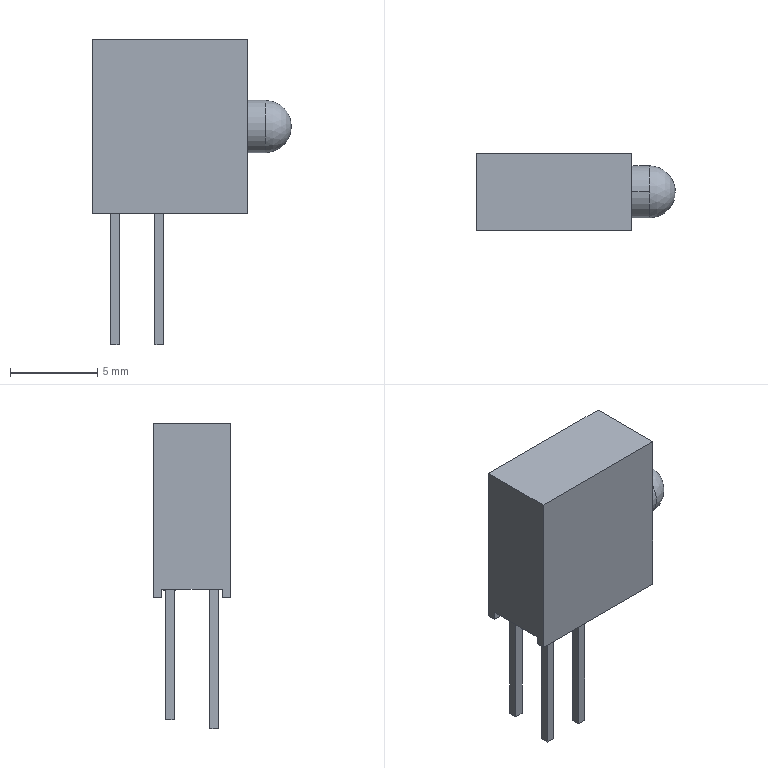Part | SolidWorks | features BaseBody 1 | 1 solid | 39 faces | box 11.4 x 4.45 x 17.5 mm | volume 402.599 mm3 | plane 34 | cylinder 4 | sphere 1 | commonest cylinder face diameters 0.707 x2 3 x2
STEP:
#1=CARTESIAN_POINT('',(107.207,42.288,40.));
#2=VERTEX_POINT('',#1);
#3=CARTESIAN_POINT('',(107.207,42.288,43.));
#4=VERTEX_POINT('',#3);
#5=CARTESIAN_POINT('',(107.207,42.288,41.5));
#6=DIRECTION('',(1.,0.,0.));
#7=DIRECTION('',(0.,0.,-1.));
#8=AXIS2_PLACEMENT_3D('',#5,#6,#7);
#9=CIRCLE('',#8,1.5);
#10=EDGE_CURVE('',#2,#4,#9,.T.);
#11=ORIENTED_EDGE('',*,*,#10,.T.);
#12=CARTESIAN_POINT('',(108.207,42.288,43.));
#13=VERTEX_POINT('',#12);
#14=CARTESIAN_POINT('',(109.807,42.288,43.));
#15=DIRECTION('',(1.,0.,0.));
#16=VECTOR('',#15,1000.);
#17=LINE('',#14,#16);
#18=EDGE_CURVE('',#4,#13,#17,.T.);
#19=ORIENTED_EDGE('',*,*,#18,.T.);
#20=CARTESIAN_POINT('',(108.207,42.288,40.));
#21=VERTEX_POINT('',#20);
#22=CARTESIAN_POINT('',(108.207,42.288,41.5));
#23=DIRECTION('',(-1.,0.,0.));
#24=DIRECTION('',(0.,0.,-1.));
#25=AXIS2_PLACEMENT_3D('',#22,#23,#24);
#26=CIRCLE('',#25,1.5);
#27=EDGE_CURVE('',#13,#21,#26,.T.);
#28=ORIENTED_EDGE('',*,*,#27,.T.);
#29=CARTESIAN_POINT('',(109.807,42.288,40.));
#30=DIRECTION('',(1.,0.,0.));
#31=VECTOR('',#30,1000.);
#32=LINE('',#29,#31);
#33=EDGE_CURVE('',#2,#21,#32,.T.);
#34=ORIENTED_EDGE('',*,*,#33,.F.);
#35=EDGE_LOOP('',(#11,#19,#28,#34));
#36=FACE_OUTER_BOUND('',#35,.T.);
#37=CARTESIAN_POINT('',(109.807,42.288,41.5));
#38=DIRECTION('',(1.,0.,0.));
#39=DIRECTION('',(0.,0.,-1.));
#40=AXIS2_PLACEMENT_3D('',#37,#38,#39);
#41=CYLINDRICAL_SURFACE('',#40,1.5);
#42=ADVANCED_FACE('',(#36),#41,.T.);
#43=CARTESIAN_POINT('',(102.481,43.558,37.));
#44=VERTEX_POINT('',#43);
#45=CARTESIAN_POINT('',(101.774,43.558,37.));
#46=VERTEX_POINT('',#45);
#47=CARTESIAN_POINT('',(102.127,43.558,37.));
#48=DIRECTION('',(0.,0.,1.));
#49=DIRECTION('',(-1.,0.,0.));
#50=AXIS2_PLACEMENT_3D('',#47,#48,#49);
#51=CIRCLE('',#50,0.3536);
#52=EDGE_CURVE('',#44,#46,#51,.T.);
#53=ORIENTED_EDGE('',*,*,#52,.F.);
#54=CARTESIAN_POINT('',(102.481,43.558,36.9));
#55=VERTEX_POINT('',#54);
#56=CARTESIAN_POINT('',(102.481,43.558,37.));
#57=DIRECTION('',(0.,0.,-1.));
#58=VECTOR('',#57,1000.);
#59=LINE('',#56,#58);
#60=EDGE_CURVE('',#44,#55,#59,.T.);
#61=ORIENTED_EDGE('',*,*,#60,.T.);
#62=CARTESIAN_POINT('',(102.377,43.808,36.9));
#63=VERTEX_POINT('',#62);
#64=CARTESIAN_POINT('',(102.127,43.558,36.9));
#65=DIRECTION('',(0.,0.,1.));
#66=DIRECTION('',(-1.,0.,0.));
#67=AXIS2_PLACEMENT_3D('',#64,#65,#66);
#68=CIRCLE('',#67,0.3536);
#69=EDGE_CURVE('',#55,#63,#68,.T.);
#70=ORIENTED_EDGE('',*,*,#69,.T.);
#71=CARTESIAN_POINT('',(101.877,43.808,36.9));
#72=VERTEX_POINT('',#71);
#73=CARTESIAN_POINT('',(102.127,43.558,36.9));
#74=DIRECTION('',(0.,0.,1.));
#75=DIRECTION('',(-1.,0.,0.));
#76=AXIS2_PLACEMENT_3D('',#73,#74,#75);
#77=CIRCLE('',#76,0.3536);
#78=EDGE_CURVE('',#63,#72,#77,.T.);
#79=ORIENTED_EDGE('',*,*,#78,.T.);
#80=CARTESIAN_POINT('',(101.774,43.558,36.9));
#81=VERTEX_POINT('',#80);
#82=CARTESIAN_POINT('',(102.127,43.558,36.9));
#83=DIRECTION('',(0.,0.,1.));
#84=DIRECTION('',(-1.,0.,0.));
#85=AXIS2_PLACEMENT_3D('',#82,#83,#84);
#86=CIRCLE('',#85,0.3536);
#87=EDGE_CURVE('',#72,#81,#86,.T.);
#88=ORIENTED_EDGE('',*,*,#87,.T.);
#89=CARTESIAN_POINT('',(101.774,43.558,37.));
#90=DIRECTION('',(0.,0.,-1.));
#91=VECTOR('',#90,1000.);
#92=LINE('',#89,#91);
#93=EDGE_CURVE('',#46,#81,#92,.T.);
#94=ORIENTED_EDGE('',*,*,#93,.F.);
#95=EDGE_LOOP('',(#53,#61,#70,#79,#88,#94));
#96=FACE_OUTER_BOUND('',#95,.T.);
#97=CARTESIAN_POINT('',(102.127,43.558,37.));
#98=DIRECTION('',(0.,0.,-1.));
#99=DIRECTION('',(-1.,0.,0.));
#100=AXIS2_PLACEMENT_3D('',#97,#98,#99);
#101=CYLINDRICAL_SURFACE('',#100,0.3536);
#102=ADVANCED_FACE('',(#96),#101,.T.);
#103=CARTESIAN_POINT('',(98.307,44.513,36.5));
#104=VERTEX_POINT('',#103);
#105=CARTESIAN_POINT('',(98.307,44.513,46.5));
#106=VERTEX_POINT('',#105);
#107=CARTESIAN_POINT('',(98.307,44.513,36.5));
#108=DIRECTION('',(0.,0.,1.));
#109=VECTOR('',#108,1000.);
#110=LINE('',#107,#109);
#111=EDGE_CURVE('',#104,#106,#110,.T.);
#112=ORIENTED_EDGE('',*,*,#111,.T.);
#113=CARTESIAN_POINT('',(107.207,44.513,46.5));
#114=VERTEX_POINT('',#113);
#115=CARTESIAN_POINT('',(98.307,44.513,46.5));
#116=DIRECTION('',(1.,0.,0.));
#117=VECTOR('',#116,1000.);
#118=LINE('',#115,#117);
#119=EDGE_CURVE('',#106,#114,#118,.T.);
#120=ORIENTED_EDGE('',*,*,#119,.T.);
#121=CARTESIAN_POINT('',(107.207,44.513,36.5));
#122=VERTEX_POINT('',#121);
#123=CARTESIAN_POINT('',(107.207,44.513,36.5));
#124=DIRECTION('',(0.,0.,-1.));
#125=VECTOR('',#124,1000.);
#126=LINE('',#123,#125);
#127=EDGE_CURVE('',#114,#122,#126,.T.);
#128=ORIENTED_EDGE('',*,*,#127,.T.);
#129=CARTESIAN_POINT('',(98.307,44.513,36.5));
#130=DIRECTION('',(-1.,0.,0.));
#131=VECTOR('',#130,1000.);
#132=LINE('',#129,#131);
#133=EDGE_CURVE('',#122,#104,#132,.T.);
#134=ORIENTED_EDGE('',*,*,#133,.T.);
#135=EDGE_LOOP('',(#112,#120,#128,#134));
#136=FACE_OUTER_BOUND('',#135,.T.);
#137=CARTESIAN_POINT('',(98.307,44.513,36.5));
#138=DIRECTION('',(0.,1.,0.));
#139=DIRECTION('',(0.,0.,1.));
#140=AXIS2_PLACEMENT_3D('',#137,#138,#139);
#141=PLANE('',#140);
#142=ADVANCED_FACE('',(#136),#141,.T.);
#143=ORIENTED_EDGE('',*,*,#119,.F.);
#144=CARTESIAN_POINT('',(98.307,40.063,46.5));
#145=VERTEX_POINT('',#144);
#146=CARTESIAN_POINT('',(98.307,44.513,46.5));
#147=DIRECTION('',(0.,1.,0.));
#148=VECTOR('',#147,1000.);
#149=LINE('',#146,#148);
#150=EDGE_CURVE('',#145,#106,#149,.T.);
#151=ORIENTED_EDGE('',*,*,#150,.F.);
#152=CARTESIAN_POINT('',(107.207,40.063,46.5));
#153=VERTEX_POINT('',#152);
#154=CARTESIAN_POINT('',(98.307,40.063,46.5));
#155=DIRECTION('',(-1.,0.,0.));
#156=VECTOR('',#155,1000.);
#157=LINE('',#154,#156);
#158=EDGE_CURVE('',#153,#145,#157,.T.);
#159=ORIENTED_EDGE('',*,*,#158,.F.);
#160=CARTESIAN_POINT('',(107.207,44.513,46.5));
#161=DIRECTION('',(0.,-1.,0.));
#162=VECTOR('',#161,1000.);
#163=LINE('',#160,#162);
#164=EDGE_CURVE('',#114,#153,#163,.T.);
#165=ORIENTED_EDGE('',*,*,#164,.F.);
#166=EDGE_LOOP('',(#143,#151,#159,#165));
#167=FACE_OUTER_BOUND('',#166,.T.);
#168=CARTESIAN_POINT('',(98.307,44.513,46.5));
#169=DIRECTION('',(0.,0.,-1.));
#170=DIRECTION('',(-1.,0.,0.));
#171=AXIS2_PLACEMENT_3D('',#168,#169,#170);
#172=PLANE('',#171);
#173=ADVANCED_FACE('',(#167),#172,.F.);
#174=CARTESIAN_POINT('',(98.307,40.063,36.5));
#175=VERTEX_POINT('',#174);
#176=CARTESIAN_POINT('',(98.307,40.063,36.5));
#177=DIRECTION('',(0.,0.,-1.));
#178=VECTOR('',#177,1000.);
#179=LINE('',#176,#178);
#180=EDGE_CURVE('',#145,#175,#179,.T.);
#181=ORIENTED_EDGE('',*,*,#180,.F.);
#182=ORIENTED_EDGE('',*,*,#150,.T.);
#183=ORIENTED_EDGE('',*,*,#111,.F.);
#184=CARTESIAN_POINT('',(98.307,44.013,36.5));
#185=VERTEX_POINT('',#184);
#186=CARTESIAN_POINT('',(98.307,44.513,36.5));
#187=DIRECTION('',(0.,1.,0.));
#188=VECTOR('',#187,1000.);
#189=LINE('',#186,#188);
#190=EDGE_CURVE('',#185,#104,#189,.T.);
#191=ORIENTED_EDGE('',*,*,#190,.F.);
#192=CARTESIAN_POINT('',(98.307,44.013,37.));
#193=VERTEX_POINT('',#192);
#194=CARTESIAN_POINT('',(98.307,44.013,37.));
#195=DIRECTION('',(0.,0.,-1.));
#196=VECTOR('',#195,1000.);
#197=LINE('',#194,#196);
#198=EDGE_CURVE('',#193,#185,#197,.T.);
#199=ORIENTED_EDGE('',*,*,#198,.F.);
#200=CARTESIAN_POINT('',(98.307,40.563,37.));
#201=VERTEX_POINT('',#200);
#202=CARTESIAN_POINT('',(98.307,44.513,37.));
#203=DIRECTION('',(0.,1.,0.));
#204=VECTOR('',#203,1000.);
#205=LINE('',#202,#204);
#206=EDGE_CURVE('',#201,#193,#205,.T.);
#207=ORIENTED_EDGE('',*,*,#206,.F.);
#208=CARTESIAN_POINT('',(98.307,40.563,36.5));
#209=VERTEX_POINT('',#208);
#210=CARTESIAN_POINT('',(98.307,40.563,35.6));
#211=DIRECTION('',(0.,0.,1.));
#212=VECTOR('',#211,1000.);
#213=LINE('',#210,#212);
#214=EDGE_CURVE('',#209,#201,#213,.T.);
#215=ORIENTED_EDGE('',*,*,#214,.F.);
#216=CARTESIAN_POINT('',(98.307,44.513,36.5));
#217=DIRECTION('',(0.,-1.,0.));
#218=VECTOR('',#217,1000.);
#219=LINE('',#216,#218);
#220=EDGE_CURVE('',#209,#175,#219,.T.);
#221=ORIENTED_EDGE('',*,*,#220,.T.);
#222=EDGE_LOOP('',(#181,#182,#183,#191,#199,#207,#215,#221));
#223=FACE_OUTER_BOUND('',#222,.T.);
#224=CARTESIAN_POINT('',(98.307,44.513,36.5));
#225=DIRECTION('',(1.,0.,0.));
#226=DIRECTION('',(0.,0.,-1.));
#227=AXIS2_PLACEMENT_3D('',#224,#225,#226);
#228=PLANE('',#227);
#229=ADVANCED_FACE('',(#223),#228,.F.);
#230=ORIENTED_EDGE('',*,*,#133,.F.);
#231=CARTESIAN_POINT('',(107.207,44.013,36.5));
#232=VERTEX_POINT('',#231);
#233=CARTESIAN_POINT('',(107.207,44.513,36.5));
#234=DIRECTION('',(0.,1.,0.));
#235=VECTOR('',#234,1000.);
#236=LINE('',#233,#235);
#237=EDGE_CURVE('',#232,#122,#236,.T.);
#238=ORIENTED_EDGE('',*,*,#237,.F.);
#239=CARTESIAN_POINT('',(107.207,44.013,36.5));
#240=DIRECTION('',(1.,0.,0.));
#241=VECTOR('',#240,1000.);
#242=LINE('',#239,#241);
#243=EDGE_CURVE('',#185,#232,#242,.T.);
#244=ORIENTED_EDGE('',*,*,#243,.F.);
#245=ORIENTED_EDGE('',*,*,#190,.T.);
#246=EDGE_LOOP('',(#230,#238,#244,#245));
#247=FACE_OUTER_BOUND('',#246,.T.);
#248=CARTESIAN_POINT('',(107.207,44.513,36.5));
#249=DIRECTION('',(0.,0.,1.));
#250=DIRECTION('',(1.,0.,0.));
#251=AXIS2_PLACEMENT_3D('',#248,#249,#250);
#252=PLANE('',#251);
#253=ADVANCED_FACE('',(#247),#252,.F.);
#254=ORIENTED_EDGE('',*,*,#10,.F.);
#255=CARTESIAN_POINT('',(107.207,42.288,41.5));
#256=DIRECTION('',(1.,0.,0.));
#257=DIRECTION('',(0.,0.,-1.));
#258=AXIS2_PLACEMENT_3D('',#255,#256,#257);
#259=CIRCLE('',#258,1.5);
#260=EDGE_CURVE('',#4,#2,#259,.T.);
#261=ORIENTED_EDGE('',*,*,#260,.F.);
#262=EDGE_LOOP('',(#254,#261));
#263=FACE_BOUND('',#262,.T.);
#264=CARTESIAN_POINT('',(107.207,40.063,36.5));
#265=VERTEX_POINT('',#264);
#266=CARTESIAN_POINT('',(107.207,40.063,46.5));
#267=DIRECTION('',(0.,0.,1.));
#268=VECTOR('',#267,1000.);
#269=LINE('',#266,#268);
#270=EDGE_CURVE('',#265,#153,#269,.T.);
#271=ORIENTED_EDGE('',*,*,#270,.F.);
#272=CARTESIAN_POINT('',(107.207,40.563,36.5));
#273=VERTEX_POINT('',#272);
#274=CARTESIAN_POINT('',(107.207,44.513,36.5));
#275=DIRECTION('',(0.,1.,0.));
#276=VECTOR('',#275,1000.);
#277=LINE('',#274,#276);
#278=EDGE_CURVE('',#265,#273,#277,.T.);
#279=ORIENTED_EDGE('',*,*,#278,.T.);
#280=CARTESIAN_POINT('',(107.207,40.563,37.));
#281=VERTEX_POINT('',#280);
#282=CARTESIAN_POINT('',(107.207,40.563,35.6));
#283=DIRECTION('',(0.,0.,-1.));
#284=VECTOR('',#283,1000.);
#285=LINE('',#282,#284);
#286=EDGE_CURVE('',#281,#273,#285,.T.);
#287=ORIENTED_EDGE('',*,*,#286,.F.);
#288=CARTESIAN_POINT('',(107.207,44.013,37.));
#289=VERTEX_POINT('',#288);
#290=CARTESIAN_POINT('',(107.207,44.513,37.));
#291=DIRECTION('',(0.,-1.,0.));
#292=VECTOR('',#291,1000.);
#293=LINE('',#290,#292);
#294=EDGE_CURVE('',#289,#281,#293,.T.);
#295=ORIENTED_EDGE('',*,*,#294,.F.);
#296=CARTESIAN_POINT('',(107.207,44.013,46.5));
#297=DIRECTION('',(0.,0.,1.));
#298=VECTOR('',#297,1000.);
#299=LINE('',#296,#298);
#300=EDGE_CURVE('',#232,#289,#299,.T.);
#301=ORIENTED_EDGE('',*,*,#300,.F.);
#302=ORIENTED_EDGE('',*,*,#237,.T.);
#303=ORIENTED_EDGE('',*,*,#127,.F.);
#304=ORIENTED_EDGE('',*,*,#164,.T.);
#305=EDGE_LOOP('',(#271,#279,#287,#295,#301,#302,#303,#304));
#306=FACE_OUTER_BOUND('',#305,.T.);
#307=CARTESIAN_POINT('',(107.207,44.513,46.5));
#308=DIRECTION('',(-1.,0.,0.));
#309=DIRECTION('',(0.,0.,1.));
#310=AXIS2_PLACEMENT_3D('',#307,#308,#309);
#311=PLANE('',#310);
#312=ADVANCED_FACE('',(#263,#306),#311,.F.);
#313=ORIENTED_EDGE('',*,*,#270,.T.);
#314=ORIENTED_EDGE('',*,*,#158,.T.);
#315=ORIENTED_EDGE('',*,*,#180,.T.);
#316=CARTESIAN_POINT('',(98.307,40.063,36.5));
#317=DIRECTION('',(-1.,0.,0.));
#318=VECTOR('',#317,1000.);
#319=LINE('',#316,#318);
#320=EDGE_CURVE('',#265,#175,#319,.T.);
#321=ORIENTED_EDGE('',*,*,#320,.F.);
#322=EDGE_LOOP('',(#313,#314,#315,#321));
#323=FACE_OUTER_BOUND('',#322,.T.);
#324=CARTESIAN_POINT('',(98.307,40.063,36.5));
#325=DIRECTION('',(0.,1.,0.));
#326=DIRECTION('',(0.,0.,1.));
#327=AXIS2_PLACEMENT_3D('',#324,#325,#326);
#328=PLANE('',#327);
#329=ADVANCED_FACE('',(#323),#328,.F.);
#330=CARTESIAN_POINT('',(102.127,43.558,37.));
#331=DIRECTION('',(0.,0.,1.));
#332=DIRECTION('',(-1.,0.,0.));
#333=AXIS2_PLACEMENT_3D('',#330,#331,#332);
#334=CIRCLE('',#333,0.3536);
#335=EDGE_CURVE('',#46,#44,#334,.T.);
#336=ORIENTED_EDGE('',*,*,#335,.T.);
#337=ORIENTED_EDGE('',*,*,#52,.T.);
#338=EDGE_LOOP('',(#336,#337));
#339=FACE_BOUND('',#338,.T.);
#340=CARTESIAN_POINT('',(99.837,43.808,37.));
#341=VERTEX_POINT('',#340);
#342=CARTESIAN_POINT('',(99.837,43.308,37.));
#343=VERTEX_POINT('',#342);
#344=CARTESIAN_POINT('',(99.837,43.808,37.));
#345=DIRECTION('',(0.,-1.,0.));
#346=VECTOR('',#345,1000.);
#347=LINE('',#344,#346);
#348=EDGE_CURVE('',#341,#343,#347,.T.);
#349=ORIENTED_EDGE('',*,*,#348,.F.);
#350=CARTESIAN_POINT('',(99.337,43.808,37.));
#351=VERTEX_POINT('',#350);
#352=CARTESIAN_POINT('',(92.707,43.808,37.));
#353=DIRECTION('',(-1.,0.,0.));
#354=VECTOR('',#353,1000.);
#355=LINE('',#352,#354);
#356=EDGE_CURVE('',#341,#351,#355,.T.);
#357=ORIENTED_EDGE('',*,*,#356,.T.);
#358=CARTESIAN_POINT('',(99.337,43.308,37.));
#359=VERTEX_POINT('',#358);
#360=CARTESIAN_POINT('',(99.337,43.558,37.));
#361=DIRECTION('',(0.,1.,0.));
#362=VECTOR('',#361,1000.);
#363=LINE('',#360,#362);
#364=EDGE_CURVE('',#359,#351,#363,.T.);
#365=ORIENTED_EDGE('',*,*,#364,.F.);
#366=CARTESIAN_POINT('',(100.857,43.308,37.));
#367=DIRECTION('',(-1.,0.,0.));
#368=VECTOR('',#367,1000.);
#369=LINE('',#366,#368);
#370=EDGE_CURVE('',#343,#359,#369,.T.);
#371=ORIENTED_EDGE('',*,*,#370,.F.);
#372=EDGE_LOOP('',(#349,#357,#365,#371));
#373=FACE_BOUND('',#372,.T.);
#374=CARTESIAN_POINT('',(99.837,41.268,37.));
#375=VERTEX_POINT('',#374);
#376=CARTESIAN_POINT('',(99.837,40.768,37.));
#377=VERTEX_POINT('',#376);
#378=CARTESIAN_POINT('',(99.837,41.268,37.));
#379=DIRECTION('',(0.,-1.,0.));
#380=VECTOR('',#379,1000.);
#381=LINE('',#378,#380);
#382=EDGE_CURVE('',#375,#377,#381,.T.);
#383=ORIENTED_EDGE('',*,*,#382,.F.);
#384=CARTESIAN_POINT('',(99.337,41.268,37.));
#385=VERTEX_POINT('',#384);
#386=CARTESIAN_POINT('',(92.707,41.268,37.));
#387=DIRECTION('',(-1.,0.,0.));
#388=VECTOR('',#387,1000.);
#389=LINE('',#386,#388);
#390=EDGE_CURVE('',#375,#385,#389,.T.);
#391=ORIENTED_EDGE('',*,*,#390,.T.);
#392=CARTESIAN_POINT('',(99.337,40.768,37.));
#393=VERTEX_POINT('',#392);
#394=CARTESIAN_POINT('',(99.337,41.268,37.));
#395=DIRECTION('',(0.,1.,0.));
#396=VECTOR('',#395,1000.);
#397=LINE('',#394,#396);
#398=EDGE_CURVE('',#393,#385,#397,.T.);
#399=ORIENTED_EDGE('',*,*,#398,.F.);
#400=CARTESIAN_POINT('',(98.307,40.768,37.));
#401=DIRECTION('',(-1.,0.,0.));
#402=VECTOR('',#401,1000.);
#403=LINE('',#400,#402);
#404=EDGE_CURVE('',#377,#393,#403,.T.);
#405=ORIENTED_EDGE('',*,*,#404,.F.);
#406=EDGE_LOOP('',(#383,#391,#399,#405));
#407=FACE_BOUND('',#406,.T.);
#408=ORIENTED_EDGE('',*,*,#206,.T.);
#409=CARTESIAN_POINT('',(92.707,44.013,37.));
#410=DIRECTION('',(1.,0.,0.));
#411=VECTOR('',#410,1000.);
#412=LINE('',#409,#411);
#413=EDGE_CURVE('',#193,#289,#412,.T.);
#414=ORIENTED_EDGE('',*,*,#413,.T.);
#415=ORIENTED_EDGE('',*,*,#294,.T.);
#416=CARTESIAN_POINT('',(92.707,40.563,37.));
#417=DIRECTION('',(-1.,0.,0.));
#418=VECTOR('',#417,1000.);
#419=LINE('',#416,#418);
#420=EDGE_CURVE('',#281,#201,#419,.T.);
#421=ORIENTED_EDGE('',*,*,#420,.T.);
#422=EDGE_LOOP('',(#408,#414,#415,#421));
#423=FACE_OUTER_BOUND('',#422,.T.);
#424=CARTESIAN_POINT('',(101.877,41.268,37.));
#425=VERTEX_POINT('',#424);
#426=CARTESIAN_POINT('',(102.377,41.268,37.));
#427=VERTEX_POINT('',#426);
#428=CARTESIAN_POINT('',(98.307,41.268,37.));
#429=DIRECTION('',(1.,0.,0.));
#430=VECTOR('',#429,1000.);
#431=LINE('',#428,#430);
#432=EDGE_CURVE('',#425,#427,#431,.T.);
#433=ORIENTED_EDGE('',*,*,#432,.F.);
#434=CARTESIAN_POINT('',(101.877,40.768,37.));
#435=VERTEX_POINT('',#434);
#436=CARTESIAN_POINT('',(101.877,40.563,37.));
#437=DIRECTION('',(0.,-1.,0.));
#438=VECTOR('',#437,1000.);
#439=LINE('',#436,#438);
#440=EDGE_CURVE('',#425,#435,#439,.T.);
#441=ORIENTED_EDGE('',*,*,#440,.T.);
#442=CARTESIAN_POINT('',(102.377,40.768,37.));
#443=VERTEX_POINT('',#442);
#444=CARTESIAN_POINT('',(98.307,40.768,37.));
#445=DIRECTION('',(1.,0.,0.));
#446=VECTOR('',#445,1000.);
#447=LINE('',#444,#446);
#448=EDGE_CURVE('',#435,#443,#447,.T.);
#449=ORIENTED_EDGE('',*,*,#448,.T.);
#450=CARTESIAN_POINT('',(102.377,41.268,37.));
#451=DIRECTION('',(0.,1.,0.));
#452=VECTOR('',#451,1000.);
#453=LINE('',#450,#452);
#454=EDGE_CURVE('',#443,#427,#453,.T.);
#455=ORIENTED_EDGE('',*,*,#454,.T.);
#456=EDGE_LOOP('',(#433,#441,#449,#455));
#457=FACE_BOUND('',#456,.T.);
#458=CARTESIAN_POINT('',(92.707,40.563,37.));
#459=DIRECTION('',(0.,0.,-1.));
#460=DIRECTION('',(-1.,0.,0.));
#461=AXIS2_PLACEMENT_3D('',#458,#459,#460);
#462=PLANE('',#461);
#463=ADVANCED_FACE('',(#339,#373,#407,#423,#457),#462,.T.);
#464=ORIENTED_EDGE('',*,*,#198,.T.);
#465=ORIENTED_EDGE('',*,*,#243,.T.);
#466=ORIENTED_EDGE('',*,*,#300,.T.);
#467=ORIENTED_EDGE('',*,*,#413,.F.);
#468=EDGE_LOOP('',(#464,#465,#466,#467));
#469=FACE_OUTER_BOUND('',#468,.T.);
#470=CARTESIAN_POINT('',(92.707,44.013,37.));
#471=DIRECTION('',(0.,-1.,0.));
#472=DIRECTION('',(0.,0.,-1.));
#473=AXIS2_PLACEMENT_3D('',#470,#471,#472);
#474=PLANE('',#473);
#475=ADVANCED_FACE('',(#469),#474,.T.);
#476=ORIENTED_EDGE('',*,*,#18,.F.);
#477=ORIENTED_EDGE('',*,*,#260,.T.);
#478=ORIENTED_EDGE('',*,*,#33,.T.);
#479=CARTESIAN_POINT('',(108.207,42.288,41.5));
#480=DIRECTION('',(-1.,0.,0.));
#481=DIRECTION('',(0.,0.,-1.));
#482=AXIS2_PLACEMENT_3D('',#479,#480,#481);
#483=CIRCLE('',#482,1.5);
#484=EDGE_CURVE('',#21,#13,#483,.T.);
#485=ORIENTED_EDGE('',*,*,#484,.T.);
#486=EDGE_LOOP('',(#476,#477,#478,#485));
#487=FACE_OUTER_BOUND('',#486,.T.);
#488=CARTESIAN_POINT('',(109.807,42.288,41.5));
#489=DIRECTION('',(1.,0.,0.));
#490=DIRECTION('',(0.,0.,-1.));
#491=AXIS2_PLACEMENT_3D('',#488,#489,#490);
#492=CYLINDRICAL_SURFACE('',#491,1.5);
#493=ADVANCED_FACE('',(#487),#492,.T.);
#494=ORIENTED_EDGE('',*,*,#320,.T.);
#495=ORIENTED_EDGE('',*,*,#220,.F.);
#496=CARTESIAN_POINT('',(107.207,40.563,36.5));
#497=DIRECTION('',(-1.,0.,0.));
#498=VECTOR('',#497,1000.);
#499=LINE('',#496,#498);
#500=EDGE_CURVE('',#273,#209,#499,.T.);
#501=ORIENTED_EDGE('',*,*,#500,.F.);
#502=ORIENTED_EDGE('',*,*,#278,.F.);
#503=EDGE_LOOP('',(#494,#495,#501,#502));
#504=FACE_OUTER_BOUND('',#503,.T.);
#505=CARTESIAN_POINT('',(107.207,44.513,36.5));
#506=DIRECTION('',(0.,0.,1.));
#507=DIRECTION('',(1.,0.,0.));
#508=AXIS2_PLACEMENT_3D('',#505,#506,#507);
#509=PLANE('',#508);
#510=ADVANCED_FACE('',(#504),#509,.F.);
#511=ORIENTED_EDGE('',*,*,#60,.F.);
#512=ORIENTED_EDGE('',*,*,#335,.F.);
#513=ORIENTED_EDGE('',*,*,#93,.T.);
#514=CARTESIAN_POINT('',(101.877,43.308,36.9));
#515=VERTEX_POINT('',#514);
#516=CARTESIAN_POINT('',(102.127,43.558,36.9));
#517=DIRECTION('',(0.,0.,1.));
#518=DIRECTION('',(-1.,0.,0.));
#519=AXIS2_PLACEMENT_3D('',#516,#517,#518);
#520=CIRCLE('',#519,0.3536);
#521=EDGE_CURVE('',#81,#515,#520,.T.);
#522=ORIENTED_EDGE('',*,*,#521,.T.);
#523=CARTESIAN_POINT('',(102.377,43.308,36.9));
#524=VERTEX_POINT('',#523);
#525=CARTESIAN_POINT('',(102.127,43.558,36.9));
#526=DIRECTION('',(0.,0.,1.));
#527=DIRECTION('',(-1.,0.,0.));
#528=AXIS2_PLACEMENT_3D('',#525,#526,#527);
#529=CIRCLE('',#528,0.3536);
#530=EDGE_CURVE('',#515,#524,#529,.T.);
#531=ORIENTED_EDGE('',*,*,#530,.T.);
#532=CARTESIAN_POINT('',(102.127,43.558,36.9));
#533=DIRECTION('',(0.,0.,1.));
#534=DIRECTION('',(-1.,0.,0.));
#535=AXIS2_PLACEMENT_3D('',#532,#533,#534);
#536=CIRCLE('',#535,0.3536);
#537=EDGE_CURVE('',#524,#55,#536,.T.);
#538=ORIENTED_EDGE('',*,*,#537,.T.);
#539=EDGE_LOOP('',(#511,#512,#513,#522,#531,#538));
#540=FACE_OUTER_BOUND('',#539,.T.);
#541=CARTESIAN_POINT('',(102.127,43.558,37.));
#542=DIRECTION('',(0.,0.,-1.));
#543=DIRECTION('',(-1.,0.,0.));
#544=AXIS2_PLACEMENT_3D('',#541,#542,#543);
#545=CYLINDRICAL_SURFACE('',#544,0.3536);
#546=ADVANCED_FACE('',(#540),#545,.T.);
#547=CARTESIAN_POINT('',(99.837,43.808,29.5));
#548=VERTEX_POINT('',#547);
#549=CARTESIAN_POINT('',(99.837,43.808,28.5));
#550=DIRECTION('',(0.,0.,-1.));
#551=VECTOR('',#550,1000.);
#552=LINE('',#549,#551);
#553=EDGE_CURVE('',#341,#548,#552,.T.);
#554=ORIENTED_EDGE('',*,*,#553,.T.);
#555=CARTESIAN_POINT('',(99.337,43.808,29.5));
#556=VERTEX_POINT('',#555);
#557=CARTESIAN_POINT('',(100.857,43.808,29.5));
#558=DIRECTION('',(-1.,0.,0.));
#559=VECTOR('',#558,1000.);
#560=LINE('',#557,#559);
#561=EDGE_CURVE('',#548,#556,#560,.T.);
#562=ORIENTED_EDGE('',*,*,#561,.T.);
#563=CARTESIAN_POINT('',(99.337,43.808,28.5));
#564=DIRECTION('',(0.,0.,1.));
#565=VECTOR('',#564,1000.);
#566=LINE('',#563,#565);
#567=EDGE_CURVE('',#556,#351,#566,.T.);
#568=ORIENTED_EDGE('',*,*,#567,.T.);
#569=ORIENTED_EDGE('',*,*,#356,.F.);
#570=EDGE_LOOP('',(#554,#562,#568,#569));
#571=FACE_OUTER_BOUND('',#570,.T.);
#572=CARTESIAN_POINT('',(100.857,43.808,28.5));
#573=DIRECTION('',(0.,1.,0.));
#574=DIRECTION('',(0.,0.,1.));
#575=AXIS2_PLACEMENT_3D('',#572,#573,#574);
#576=PLANE('',#575);
#577=ADVANCED_FACE('',(#571),#576,.T.);
#578=CARTESIAN_POINT('',(99.337,41.268,29.));
#579=VERTEX_POINT('',#578);
#580=CARTESIAN_POINT('',(99.837,41.268,29.));
#581=VERTEX_POINT('',#580);
#582=CARTESIAN_POINT('',(98.307,41.268,29.));
#583=DIRECTION('',(1.,0.,0.));
#584=VECTOR('',#583,1000.);
#585=LINE('',#582,#584);
#586=EDGE_CURVE('',#579,#581,#585,.T.);
#587=ORIENTED_EDGE('',*,*,#586,.F.);
#588=CARTESIAN_POINT('',(99.337,41.268,36.5));
#589=DIRECTION('',(0.,0.,-1.));
#590=VECTOR('',#589,1000.);
#591=LINE('',#588,#590);
#592=EDGE_CURVE('',#385,#579,#591,.T.);
#593=ORIENTED_EDGE('',*,*,#592,.F.);
#594=ORIENTED_EDGE('',*,*,#390,.F.);
#595=CARTESIAN_POINT('',(99.837,41.268,36.5));
#596=DIRECTION('',(0.,0.,1.));
#597=VECTOR('',#596,1000.);
#598=LINE('',#595,#597);
#599=EDGE_CURVE('',#581,#375,#598,.T.);
#600=ORIENTED_EDGE('',*,*,#599,.F.);
#601=EDGE_LOOP('',(#587,#593,#594,#600));
#602=FACE_OUTER_BOUND('',#601,.T.);
#603=CARTESIAN_POINT('',(98.307,41.268,36.5));
#604=DIRECTION('',(0.,-1.,0.));
#605=DIRECTION('',(0.,0.,-1.));
#606=AXIS2_PLACEMENT_3D('',#603,#604,#605);
#607=PLANE('',#606);
#608=ADVANCED_FACE('',(#602),#607,.F.);
#609=ORIENTED_EDGE('',*,*,#214,.T.);
#610=ORIENTED_EDGE('',*,*,#420,.F.);
#611=ORIENTED_EDGE('',*,*,#286,.T.);
#612=ORIENTED_EDGE('',*,*,#500,.T.);
#613=EDGE_LOOP('',(#609,#610,#611,#612));
#614=FACE_OUTER_BOUND('',#613,.T.);
#615=CARTESIAN_POINT('',(92.707,40.563,35.6));
#616=DIRECTION('',(0.,1.,0.));
#617=DIRECTION('',(0.,0.,1.));
#618=AXIS2_PLACEMENT_3D('',#615,#616,#617);
#619=PLANE('',#618);
#620=ADVANCED_FACE('',(#614),#619,.T.);
#621=CARTESIAN_POINT('',(101.877,40.768,29.));
#622=VERTEX_POINT('',#621);
#623=CARTESIAN_POINT('',(101.877,41.268,29.));
#624=VERTEX_POINT('',#623);
#625=CARTESIAN_POINT('',(101.877,41.268,29.));
#626=DIRECTION('',(0.,1.,0.));
#627=VECTOR('',#626,1000.);
#628=LINE('',#625,#627);
#629=EDGE_CURVE('',#622,#624,#628,.T.);
#630=ORIENTED_EDGE('',*,*,#629,.F.);
#631=CARTESIAN_POINT('',(101.877,40.768,28.5));
#632=DIRECTION('',(0.,0.,-1.));
#633=VECTOR('',#632,1000.);
#634=LINE('',#631,#633);
#635=EDGE_CURVE('',#435,#622,#634,.T.);
#636=ORIENTED_EDGE('',*,*,#635,.F.);
#637=ORIENTED_EDGE('',*,*,#440,.F.);
#638=CARTESIAN_POINT('',(101.877,41.268,28.5));
#639=DIRECTION('',(0.,0.,1.));
#640=VECTOR('',#639,1000.);
#641=LINE('',#638,#640);
#642=EDGE_CURVE('',#624,#425,#641,.T.);
#643=ORIENTED_EDGE('',*,*,#642,.F.);
#644=EDGE_LOOP('',(#630,#636,#637,#643));
#645=FACE_OUTER_BOUND('',#644,.T.);
#646=CARTESIAN_POINT('',(101.877,41.268,28.5));
#647=DIRECTION('',(1.,0.,0.));
#648=DIRECTION('',(0.,0.,-1.));
#649=AXIS2_PLACEMENT_3D('',#646,#647,#648);
#650=PLANE('',#649);
#651=ADVANCED_FACE('',(#645),#650,.F.);
#652=ORIENTED_EDGE('',*,*,#484,.F.);
#653=ORIENTED_EDGE('',*,*,#27,.F.);
#654=EDGE_LOOP('',(#652,#653));
#655=FACE_OUTER_BOUND('',#654,.T.);
#656=CARTESIAN_POINT('',(108.207,42.288,41.5));
#657=DIRECTION('',(-1.,0.,0.));
#658=DIRECTION('',(0.,1.,0.));
#659=AXIS2_PLACEMENT_3D('',#656,#657,#658);
#660=SPHERICAL_SURFACE('',#659,1.5);
#661=ADVANCED_FACE('',(#655),#660,.T.);
#662=CARTESIAN_POINT('',(101.877,43.558,36.9));
#663=DIRECTION('',(0.,-1.,0.));
#664=VECTOR('',#663,1000.);
#665=LINE('',#662,#664);
#666=EDGE_CURVE('',#72,#515,#665,.T.);
#667=ORIENTED_EDGE('',*,*,#666,.T.);
#668=ORIENTED_EDGE('',*,*,#521,.F.);
#669=ORIENTED_EDGE('',*,*,#87,.F.);
#670=EDGE_LOOP('',(#667,#668,#669));
#671=FACE_OUTER_BOUND('',#670,.T.);
#672=CARTESIAN_POINT('',(102.127,43.558,36.9));
#673=DIRECTION('',(0.,0.,-1.));
#674=DIRECTION('',(-1.,0.,0.));
#675=AXIS2_PLACEMENT_3D('',#672,#673,#674);
#676=PLANE('',#675);
#677=ADVANCED_FACE('',(#671),#676,.T.);
#678=ORIENTED_EDGE('',*,*,#78,.F.);
#679=CARTESIAN_POINT('',(100.857,43.808,36.9));
#680=DIRECTION('',(1.,0.,0.));
#681=VECTOR('',#680,1000.);
#682=LINE('',#679,#681);
#683=EDGE_CURVE('',#72,#63,#682,.T.);
#684=ORIENTED_EDGE('',*,*,#683,.F.);
#685=EDGE_LOOP('',(#678,#684));
#686=FACE_OUTER_BOUND('',#685,.T.);
#687=CARTESIAN_POINT('',(102.127,43.558,36.9));
#688=DIRECTION('',(0.,0.,-1.));
#689=DIRECTION('',(-1.,0.,0.));
#690=AXIS2_PLACEMENT_3D('',#687,#688,#689);
#691=PLANE('',#690);
#692=ADVANCED_FACE('',(#686),#691,.T.);
#693=CARTESIAN_POINT('',(102.377,43.558,36.9));
#694=DIRECTION('',(0.,-1.,0.));
#695=VECTOR('',#694,1000.);
#696=LINE('',#693,#695);
#697=EDGE_CURVE('',#63,#524,#696,.T.);
#698=ORIENTED_EDGE('',*,*,#697,.F.);
#699=ORIENTED_EDGE('',*,*,#69,.F.);
#700=ORIENTED_EDGE('',*,*,#537,.F.);
#701=EDGE_LOOP('',(#698,#699,#700));
#702=FACE_OUTER_BOUND('',#701,.T.);
#703=CARTESIAN_POINT('',(102.127,43.558,36.9));
#704=DIRECTION('',(0.,0.,-1.));
#705=DIRECTION('',(-1.,0.,0.));
#706=AXIS2_PLACEMENT_3D('',#703,#704,#705);
#707=PLANE('',#706);
#708=ADVANCED_FACE('',(#702),#707,.T.);
#709=ORIENTED_EDGE('',*,*,#530,.F.);
#710=CARTESIAN_POINT('',(100.857,43.308,36.9));
#711=DIRECTION('',(-1.,0.,0.));
#712=VECTOR('',#711,1000.);
#713=LINE('',#710,#712);
#714=EDGE_CURVE('',#524,#515,#713,.T.);
#715=ORIENTED_EDGE('',*,*,#714,.F.);
#716=EDGE_LOOP('',(#709,#715));
#717=FACE_OUTER_BOUND('',#716,.T.);
#718=CARTESIAN_POINT('',(102.127,43.558,36.9));
#719=DIRECTION('',(0.,0.,-1.));
#720=DIRECTION('',(-1.,0.,0.));
#721=AXIS2_PLACEMENT_3D('',#718,#719,#720);
#722=PLANE('',#721);
#723=ADVANCED_FACE('',(#717),#722,.T.);
#724=ORIENTED_EDGE('',*,*,#561,.F.);
#725=CARTESIAN_POINT('',(99.837,43.308,29.5));
#726=VERTEX_POINT('',#725);
#727=CARTESIAN_POINT('',(99.837,43.558,29.5));
#728=DIRECTION('',(0.,-1.,0.));
#729=VECTOR('',#728,1000.);
#730=LINE('',#727,#729);
#731=EDGE_CURVE('',#548,#726,#730,.T.);
#732=ORIENTED_EDGE('',*,*,#731,.T.);
#733=CARTESIAN_POINT('',(99.337,43.308,29.5));
#734=VERTEX_POINT('',#733);
#735=CARTESIAN_POINT('',(100.857,43.308,29.5));
#736=DIRECTION('',(1.,0.,0.));
#737=VECTOR('',#736,1000.);
#738=LINE('',#735,#737);
#739=EDGE_CURVE('',#734,#726,#738,.T.);
#740=ORIENTED_EDGE('',*,*,#739,.F.);
#741=CARTESIAN_POINT('',(99.337,43.558,29.5));
#742=DIRECTION('',(0.,1.,0.));
#743=VECTOR('',#742,1000.);
#744=LINE('',#741,#743);
#745=EDGE_CURVE('',#734,#556,#744,.T.);
#746=ORIENTED_EDGE('',*,*,#745,.T.);
#747=EDGE_LOOP('',(#724,#732,#740,#746));
#748=FACE_OUTER_BOUND('',#747,.T.);
#749=CARTESIAN_POINT('',(100.857,43.558,29.5));
#750=DIRECTION('',(0.,0.,-1.));
#751=DIRECTION('',(-1.,0.,0.));
#752=AXIS2_PLACEMENT_3D('',#749,#750,#751);
#753=PLANE('',#752);
#754=ADVANCED_FACE('',(#748),#753,.T.);
#755=ORIENTED_EDGE('',*,*,#553,.F.);
#756=ORIENTED_EDGE('',*,*,#348,.T.);
#757=CARTESIAN_POINT('',(99.837,43.308,28.5));
#758=DIRECTION('',(0.,0.,-1.));
#759=VECTOR('',#758,1000.);
#760=LINE('',#757,#759);
#761=EDGE_CURVE('',#343,#726,#760,.T.);
#762=ORIENTED_EDGE('',*,*,#761,.T.);
#763=ORIENTED_EDGE('',*,*,#731,.F.);
#764=EDGE_LOOP('',(#755,#756,#762,#763));
#765=FACE_OUTER_BOUND('',#764,.T.);
#766=CARTESIAN_POINT('',(99.837,43.808,28.5));
#767=DIRECTION('',(1.,0.,0.));
#768=DIRECTION('',(0.,0.,-1.));
#769=AXIS2_PLACEMENT_3D('',#766,#767,#768);
#770=PLANE('',#769);
#771=ADVANCED_FACE('',(#765),#770,.T.);
#772=ORIENTED_EDGE('',*,*,#745,.F.);
#773=CARTESIAN_POINT('',(99.337,43.308,28.5));
#774=DIRECTION('',(0.,0.,1.));
#775=VECTOR('',#774,1000.);
#776=LINE('',#773,#775);
#777=EDGE_CURVE('',#734,#359,#776,.T.);
#778=ORIENTED_EDGE('',*,*,#777,.T.);
#779=ORIENTED_EDGE('',*,*,#364,.T.);
#780=ORIENTED_EDGE('',*,*,#567,.F.);
#781=EDGE_LOOP('',(#772,#778,#779,#780));
#782=FACE_OUTER_BOUND('',#781,.T.);
#783=CARTESIAN_POINT('',(99.337,43.558,28.5));
#784=DIRECTION('',(-1.,0.,0.));
#785=DIRECTION('',(0.,0.,1.));
#786=AXIS2_PLACEMENT_3D('',#783,#784,#785);
#787=PLANE('',#786);
#788=ADVANCED_FACE('',(#782),#787,.T.);
#789=ORIENTED_EDGE('',*,*,#599,.T.);
#790=ORIENTED_EDGE('',*,*,#382,.T.);
#791=CARTESIAN_POINT('',(99.837,40.768,29.));
#792=VERTEX_POINT('',#791);
#793=CARTESIAN_POINT('',(99.837,40.768,28.5));
#794=DIRECTION('',(0.,0.,-1.));
#795=VECTOR('',#794,1000.);
#796=LINE('',#793,#795);
#797=EDGE_CURVE('',#377,#792,#796,.T.);
#798=ORIENTED_EDGE('',*,*,#797,.T.);
#799=CARTESIAN_POINT('',(99.837,41.268,29.));
#800=DIRECTION('',(0.,1.,0.));
#801=VECTOR('',#800,1000.);
#802=LINE('',#799,#801);
#803=EDGE_CURVE('',#792,#581,#802,.T.);
#804=ORIENTED_EDGE('',*,*,#803,.T.);
#805=EDGE_LOOP('',(#789,#790,#798,#804));
#806=FACE_OUTER_BOUND('',#805,.T.);
#807=CARTESIAN_POINT('',(99.837,41.268,28.5));
#808=DIRECTION('',(1.,0.,0.));
#809=DIRECTION('',(0.,0.,-1.));
#810=AXIS2_PLACEMENT_3D('',#807,#808,#809);
#811=PLANE('',#810);
#812=ADVANCED_FACE('',(#806),#811,.T.);
#813=CARTESIAN_POINT('',(99.337,40.768,29.));
#814=VERTEX_POINT('',#813);
#815=CARTESIAN_POINT('',(99.337,40.768,29.));
#816=DIRECTION('',(-1.,0.,0.));
#817=VECTOR('',#816,1000.);
#818=LINE('',#815,#817);
#819=EDGE_CURVE('',#792,#814,#818,.T.);
#820=ORIENTED_EDGE('',*,*,#819,.T.);
#821=CARTESIAN_POINT('',(99.337,41.268,29.));
#822=DIRECTION('',(0.,1.,0.));
#823=VECTOR('',#822,1000.);
#824=LINE('',#821,#823);
#825=EDGE_CURVE('',#814,#579,#824,.T.);
#826=ORIENTED_EDGE('',*,*,#825,.T.);
#827=ORIENTED_EDGE('',*,*,#586,.T.);
#828=ORIENTED_EDGE('',*,*,#803,.F.);
#829=EDGE_LOOP('',(#820,#826,#827,#828));
#830=FACE_OUTER_BOUND('',#829,.T.);
#831=CARTESIAN_POINT('',(99.337,41.268,29.));
#832=DIRECTION('',(0.,0.,-1.));
#833=DIRECTION('',(-1.,0.,0.));
#834=AXIS2_PLACEMENT_3D('',#831,#832,#833);
#835=PLANE('',#834);
#836=ADVANCED_FACE('',(#830),#835,.T.);
#837=CARTESIAN_POINT('',(99.337,40.768,36.5));
#838=DIRECTION('',(0.,0.,1.));
#839=VECTOR('',#838,1000.);
#840=LINE('',#837,#839);
#841=EDGE_CURVE('',#814,#393,#840,.T.);
#842=ORIENTED_EDGE('',*,*,#841,.T.);
#843=ORIENTED_EDGE('',*,*,#398,.T.);
#844=ORIENTED_EDGE('',*,*,#592,.T.);
#845=ORIENTED_EDGE('',*,*,#825,.F.);
#846=EDGE_LOOP('',(#842,#843,#844,#845));
#847=FACE_OUTER_BOUND('',#846,.T.);
#848=CARTESIAN_POINT('',(99.337,41.268,36.5));
#849=DIRECTION('',(-1.,0.,0.));
#850=DIRECTION('',(0.,0.,1.));
#851=AXIS2_PLACEMENT_3D('',#848,#849,#850);
#852=PLANE('',#851);
#853=ADVANCED_FACE('',(#847),#852,.T.);
#854=ORIENTED_EDGE('',*,*,#642,.T.);
#855=ORIENTED_EDGE('',*,*,#432,.T.);
#856=CARTESIAN_POINT('',(102.377,41.268,29.));
#857=VERTEX_POINT('',#856);
#858=CARTESIAN_POINT('',(102.377,41.268,36.5));
#859=DIRECTION('',(0.,0.,-1.));
#860=VECTOR('',#859,1000.);
#861=LINE('',#858,#860);
#862=EDGE_CURVE('',#427,#857,#861,.T.);
#863=ORIENTED_EDGE('',*,*,#862,.T.);
#864=CARTESIAN_POINT('',(98.307,41.268,29.));
#865=DIRECTION('',(-1.,0.,0.));
#866=VECTOR('',#865,1000.);
#867=LINE('',#864,#866);
#868=EDGE_CURVE('',#857,#624,#867,.T.);
#869=ORIENTED_EDGE('',*,*,#868,.T.);
#870=EDGE_LOOP('',(#854,#855,#863,#869));
#871=FACE_OUTER_BOUND('',#870,.T.);
#872=CARTESIAN_POINT('',(98.307,41.268,36.5));
#873=DIRECTION('',(0.,1.,0.));
#874=DIRECTION('',(0.,0.,1.));
#875=AXIS2_PLACEMENT_3D('',#872,#873,#874);
#876=PLANE('',#875);
#877=ADVANCED_FACE('',(#871),#876,.T.);
#878=ORIENTED_EDGE('',*,*,#868,.F.);
#879=CARTESIAN_POINT('',(102.377,40.768,29.));
#880=VERTEX_POINT('',#879);
#881=CARTESIAN_POINT('',(102.377,41.268,29.));
#882=DIRECTION('',(0.,1.,0.));
#883=VECTOR('',#882,1000.);
#884=LINE('',#881,#883);
#885=EDGE_CURVE('',#880,#857,#884,.T.);
#886=ORIENTED_EDGE('',*,*,#885,.F.);
#887=CARTESIAN_POINT('',(102.377,40.768,29.));
#888=DIRECTION('',(1.,0.,0.));
#889=VECTOR('',#888,1000.);
#890=LINE('',#887,#889);
#891=EDGE_CURVE('',#622,#880,#890,.T.);
#892=ORIENTED_EDGE('',*,*,#891,.F.);
#893=ORIENTED_EDGE('',*,*,#629,.T.);
#894=EDGE_LOOP('',(#878,#886,#892,#893));
#895=FACE_OUTER_BOUND('',#894,.T.);
#896=CARTESIAN_POINT('',(102.377,41.268,29.));
#897=DIRECTION('',(0.,0.,1.));
#898=DIRECTION('',(1.,0.,0.));
#899=AXIS2_PLACEMENT_3D('',#896,#897,#898);
#900=PLANE('',#899);
#901=ADVANCED_FACE('',(#895),#900,.F.);
#902=ORIENTED_EDGE('',*,*,#891,.T.);
#903=CARTESIAN_POINT('',(102.377,40.768,36.5));
#904=DIRECTION('',(0.,0.,-1.));
#905=VECTOR('',#904,1000.);
#906=LINE('',#903,#905);
#907=EDGE_CURVE('',#443,#880,#906,.T.);
#908=ORIENTED_EDGE('',*,*,#907,.F.);
#909=ORIENTED_EDGE('',*,*,#448,.F.);
#910=ORIENTED_EDGE('',*,*,#635,.T.);
#911=EDGE_LOOP('',(#902,#908,#909,#910));
#912=FACE_OUTER_BOUND('',#911,.T.);
#913=CARTESIAN_POINT('',(98.307,40.768,36.5));
#914=DIRECTION('',(0.,1.,0.));
#915=DIRECTION('',(0.,0.,1.));
#916=AXIS2_PLACEMENT_3D('',#913,#914,#915);
#917=PLANE('',#916);
#918=ADVANCED_FACE('',(#912),#917,.F.);
#919=CARTESIAN_POINT('',(101.877,43.808,29.5));
#920=VERTEX_POINT('',#919);
#921=CARTESIAN_POINT('',(101.877,43.808,28.5));
#922=DIRECTION('',(0.,0.,1.));
#923=VECTOR('',#922,1000.);
#924=LINE('',#921,#923);
#925=EDGE_CURVE('',#920,#72,#924,.T.);
#926=ORIENTED_EDGE('',*,*,#925,.F.);
#927=CARTESIAN_POINT('',(101.877,43.308,29.5));
#928=VERTEX_POINT('',#927);
#929=CARTESIAN_POINT('',(101.877,43.808,29.5));
#930=DIRECTION('',(0.,1.,0.));
#931=VECTOR('',#930,1000.);
#932=LINE('',#929,#931);
#933=EDGE_CURVE('',#928,#920,#932,.T.);
#934=ORIENTED_EDGE('',*,*,#933,.F.);
#935=CARTESIAN_POINT('',(101.877,43.308,28.5));
#936=DIRECTION('',(0.,0.,-1.));
#937=VECTOR('',#936,1000.);
#938=LINE('',#935,#937);
#939=EDGE_CURVE('',#515,#928,#938,.T.);
#940=ORIENTED_EDGE('',*,*,#939,.F.);
#941=ORIENTED_EDGE('',*,*,#666,.F.);
#942=EDGE_LOOP('',(#926,#934,#940,#941));
#943=FACE_OUTER_BOUND('',#942,.T.);
#944=CARTESIAN_POINT('',(101.877,43.808,28.5));
#945=DIRECTION('',(1.,0.,0.));
#946=DIRECTION('',(0.,0.,-1.));
#947=AXIS2_PLACEMENT_3D('',#944,#945,#946);
#948=PLANE('',#947);
#949=ADVANCED_FACE('',(#943),#948,.F.);
#950=ORIENTED_EDGE('',*,*,#739,.T.);
#951=ORIENTED_EDGE('',*,*,#761,.F.);
#952=ORIENTED_EDGE('',*,*,#370,.T.);
#953=ORIENTED_EDGE('',*,*,#777,.F.);
#954=EDGE_LOOP('',(#950,#951,#952,#953));
#955=FACE_OUTER_BOUND('',#954,.T.);
#956=CARTESIAN_POINT('',(100.857,43.308,28.5));
#957=DIRECTION('',(0.,-1.,0.));
#958=DIRECTION('',(0.,0.,-1.));
#959=AXIS2_PLACEMENT_3D('',#956,#957,#958);
#960=PLANE('',#959);
#961=ADVANCED_FACE('',(#955),#960,.T.);
#962=ORIENTED_EDGE('',*,*,#797,.F.);
#963=ORIENTED_EDGE('',*,*,#404,.T.);
#964=ORIENTED_EDGE('',*,*,#841,.F.);
#965=ORIENTED_EDGE('',*,*,#819,.F.);
#966=EDGE_LOOP('',(#962,#963,#964,#965));
#967=FACE_OUTER_BOUND('',#966,.T.);
#968=CARTESIAN_POINT('',(98.307,40.768,36.5));
#969=DIRECTION('',(0.,-1.,0.));
#970=DIRECTION('',(0.,0.,-1.));
#971=AXIS2_PLACEMENT_3D('',#968,#969,#970);
#972=PLANE('',#971);
#973=ADVANCED_FACE('',(#967),#972,.T.);
#974=ORIENTED_EDGE('',*,*,#885,.T.);
#975=ORIENTED_EDGE('',*,*,#862,.F.);
#976=ORIENTED_EDGE('',*,*,#454,.F.);
#977=ORIENTED_EDGE('',*,*,#907,.T.);
#978=EDGE_LOOP('',(#974,#975,#976,#977));
#979=FACE_OUTER_BOUND('',#978,.T.);
#980=CARTESIAN_POINT('',(102.377,41.268,36.5));
#981=DIRECTION('',(-1.,0.,0.));
#982=DIRECTION('',(0.,0.,1.));
#983=AXIS2_PLACEMENT_3D('',#980,#981,#982);
#984=PLANE('',#983);
#985=ADVANCED_FACE('',(#979),#984,.F.);
#986=ORIENTED_EDGE('',*,*,#683,.T.);
#987=CARTESIAN_POINT('',(102.377,43.808,29.5));
#988=VERTEX_POINT('',#987);
#989=CARTESIAN_POINT('',(102.377,43.808,28.5));
#990=DIRECTION('',(0.,0.,-1.));
#991=VECTOR('',#990,1000.);
#992=LINE('',#989,#991);
#993=EDGE_CURVE('',#63,#988,#992,.T.);
#994=ORIENTED_EDGE('',*,*,#993,.T.);
#995=CARTESIAN_POINT('',(100.857,43.808,29.5));
#996=DIRECTION('',(-1.,0.,0.));
#997=VECTOR('',#996,1000.);
#998=LINE('',#995,#997);
#999=EDGE_CURVE('',#988,#920,#998,.T.);
#1000=ORIENTED_EDGE('',*,*,#999,.T.);
#1001=ORIENTED_EDGE('',*,*,#925,.T.);
#1002=EDGE_LOOP('',(#986,#994,#1000,#1001));
#1003=FACE_OUTER_BOUND('',#1002,.T.);
#1004=CARTESIAN_POINT('',(100.857,43.808,28.5));
#1005=DIRECTION('',(0.,1.,0.));
#1006=DIRECTION('',(0.,0.,1.));
#1007=AXIS2_PLACEMENT_3D('',#1004,#1005,#1006);
#1008=PLANE('',#1007);
#1009=ADVANCED_FACE('',(#1003),#1008,.T.);
#1010=ORIENTED_EDGE('',*,*,#933,.T.);
#1011=ORIENTED_EDGE('',*,*,#999,.F.);
#1012=CARTESIAN_POINT('',(102.377,43.308,29.5));
#1013=VERTEX_POINT('',#1012);
#1014=CARTESIAN_POINT('',(102.377,43.558,29.5));
#1015=DIRECTION('',(0.,-1.,0.));
#1016=VECTOR('',#1015,1000.);
#1017=LINE('',#1014,#1016);
#1018=EDGE_CURVE('',#988,#1013,#1017,.T.);
#1019=ORIENTED_EDGE('',*,*,#1018,.T.);
#1020=CARTESIAN_POINT('',(100.857,43.308,29.5));
#1021=DIRECTION('',(-1.,0.,0.));
#1022=VECTOR('',#1021,1000.);
#1023=LINE('',#1020,#1022);
#1024=EDGE_CURVE('',#1013,#928,#1023,.T.);
#1025=ORIENTED_EDGE('',*,*,#1024,.T.);
#1026=EDGE_LOOP('',(#1010,#1011,#1019,#1025));
#1027=FACE_OUTER_BOUND('',#1026,.T.);
#1028=CARTESIAN_POINT('',(100.857,43.558,29.5));
#1029=DIRECTION('',(0.,0.,-1.));
#1030=DIRECTION('',(-1.,0.,0.));
#1031=AXIS2_PLACEMENT_3D('',#1028,#1029,#1030);
#1032=PLANE('',#1031);
#1033=ADVANCED_FACE('',(#1027),#1032,.T.);
#1034=ORIENTED_EDGE('',*,*,#714,.T.);
#1035=ORIENTED_EDGE('',*,*,#939,.T.);
#1036=ORIENTED_EDGE('',*,*,#1024,.F.);
#1037=CARTESIAN_POINT('',(102.377,43.308,28.5));
#1038=DIRECTION('',(0.,0.,1.));
#1039=VECTOR('',#1038,1000.);
#1040=LINE('',#1037,#1039);
#1041=EDGE_CURVE('',#1013,#524,#1040,.T.);
#1042=ORIENTED_EDGE('',*,*,#1041,.T.);
#1043=EDGE_LOOP('',(#1034,#1035,#1036,#1042));
#1044=FACE_OUTER_BOUND('',#1043,.T.);
#1045=CARTESIAN_POINT('',(100.857,43.308,28.5));
#1046=DIRECTION('',(0.,-1.,0.));
#1047=DIRECTION('',(0.,0.,-1.));
#1048=AXIS2_PLACEMENT_3D('',#1045,#1046,#1047);
#1049=PLANE('',#1048);
#1050=ADVANCED_FACE('',(#1044),#1049,.T.);
#1051=ORIENTED_EDGE('',*,*,#697,.T.);
#1052=ORIENTED_EDGE('',*,*,#1041,.F.);
#1053=ORIENTED_EDGE('',*,*,#1018,.F.);
#1054=ORIENTED_EDGE('',*,*,#993,.F.);
#1055=EDGE_LOOP('',(#1051,#1052,#1053,#1054));
#1056=FACE_OUTER_BOUND('',#1055,.T.);
#1057=CARTESIAN_POINT('',(102.377,43.558,28.5));
#1058=DIRECTION('',(1.,0.,0.));
#1059=DIRECTION('',(0.,0.,-1.));
#1060=AXIS2_PLACEMENT_3D('',#1057,#1058,#1059);
#1061=PLANE('',#1060);
#1062=ADVANCED_FACE('',(#1056),#1061,.T.);
#1063=CLOSED_SHELL('',(#42,#102,#142,#173,#229,#253,#312,#329,#463,#475,#493,#510,#546,#577,#608,#620,#651,#661,#677,#692,#708,#723,#754,#771,#788,#812,#836,#853,#877,#901,#918,#949,#961,#973,#985,#1009,#1033,#1050,#1062));
#1064=MANIFOLD_SOLID_BREP('',#1063);
#1065=CARTESIAN_POINT('',(0.,0.,0.));
#1066=DIRECTION('',(0.,0.,1.));
#1067=DIRECTION('',(1.,0.,0.));
#1068=AXIS2_PLACEMENT_3D('',#1065,#1066,#1067);
#1069=(LENGTH_UNIT()NAMED_UNIT(*)SI_UNIT(.MILLI.,.METRE.));
#1070=UNCERTAINTY_MEASURE_WITH_UNIT(LENGTH_MEASURE(0.00001),#1069,'','');
#1071=(NAMED_UNIT(*)PLANE_ANGLE_UNIT()SI_UNIT($,.RADIAN.));
#1072=(NAMED_UNIT(*)SI_UNIT($,.STERADIAN.)SOLID_ANGLE_UNIT());
#1073=(GEOMETRIC_REPRESENTATION_CONTEXT(3)GLOBAL_UNCERTAINTY_ASSIGNED_CONTEXT((#1070))GLOBAL_UNIT_ASSIGNED_CONTEXT((#1069,#1071,#1072))REPRESENTATION_CONTEXT('',''));
#1074=ADVANCED_BREP_SHAPE_REPRESENTATION('',(#1064,#1068),#1073);